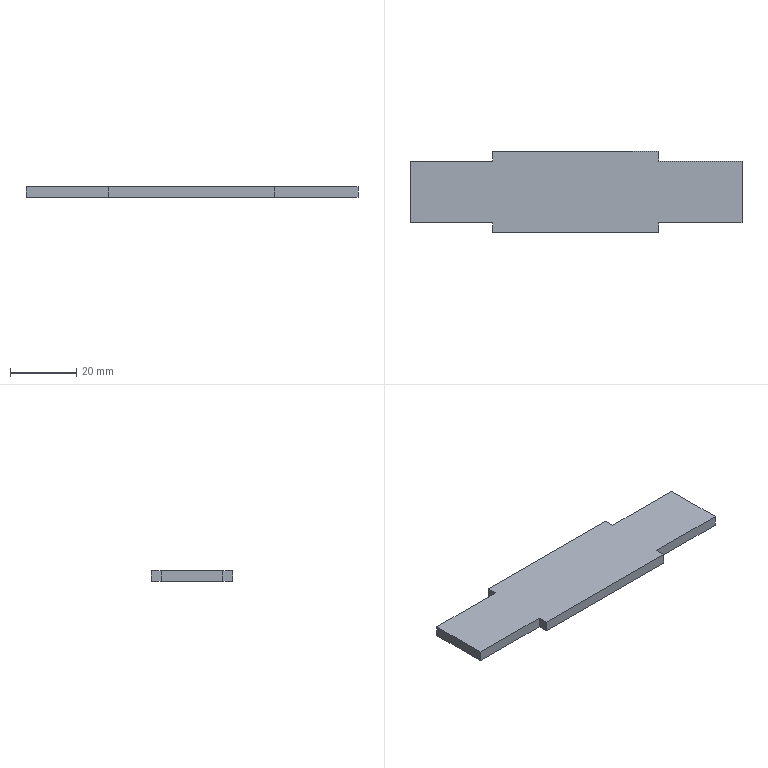Part | SolidWorks | features FlatPattern 1, SMBaseFlange 1, SheetMetal 1 | 1 solid | 14 faces | box 100 x 24.6 x 3.2 mm | volume 6912 mm3 | plane 14
STEP:
#1=CARTESIAN_POINT('',(-70.,-18.6,0.));
#2=VERTEX_POINT('',#1);
#3=CARTESIAN_POINT('',(-70.,0.,0.));
#4=VERTEX_POINT('',#3);
#5=CARTESIAN_POINT('',(-70.,0.,0.));
#6=DIRECTION('',(0.,1.,0.));
#7=VECTOR('',#6,1000.);
#8=LINE('',#5,#7);
#9=EDGE_CURVE('',#2,#4,#8,.T.);
#10=ORIENTED_EDGE('',*,*,#9,.F.);
#11=CARTESIAN_POINT('',(-70.,-18.6,-3.2));
#12=VERTEX_POINT('',#11);
#13=CARTESIAN_POINT('',(-70.,-18.6,-3.2));
#14=DIRECTION('',(0.,0.,1.));
#15=VECTOR('',#14,1000.);
#16=LINE('',#13,#15);
#17=EDGE_CURVE('',#12,#2,#16,.T.);
#18=ORIENTED_EDGE('',*,*,#17,.F.);
#19=CARTESIAN_POINT('',(-70.,0.,-3.2));
#20=VERTEX_POINT('',#19);
#21=CARTESIAN_POINT('',(-70.,0.,-3.2));
#22=DIRECTION('',(0.,1.,0.));
#23=VECTOR('',#22,1000.);
#24=LINE('',#21,#23);
#25=EDGE_CURVE('',#12,#20,#24,.T.);
#26=ORIENTED_EDGE('',*,*,#25,.T.);
#27=CARTESIAN_POINT('',(-70.,0.,-3.2));
#28=DIRECTION('',(0.,0.,1.));
#29=VECTOR('',#28,1000.);
#30=LINE('',#27,#29);
#31=EDGE_CURVE('',#20,#4,#30,.T.);
#32=ORIENTED_EDGE('',*,*,#31,.T.);
#33=EDGE_LOOP('',(#10,#18,#26,#32));
#34=FACE_OUTER_BOUND('',#33,.T.);
#35=CARTESIAN_POINT('',(-70.,0.,-3.2));
#36=DIRECTION('',(1.,0.,0.));
#37=DIRECTION('',(0.,0.,-1.));
#38=AXIS2_PLACEMENT_3D('',#35,#36,#37);
#39=PLANE('',#38);
#40=ADVANCED_FACE('',(#34),#39,.T.);
#41=CARTESIAN_POINT('',(-95.,-18.6,0.));
#42=VERTEX_POINT('',#41);
#43=CARTESIAN_POINT('',(-70.,-18.6,0.));
#44=DIRECTION('',(1.,0.,0.));
#45=VECTOR('',#44,1000.);
#46=LINE('',#43,#45);
#47=EDGE_CURVE('',#42,#2,#46,.T.);
#48=ORIENTED_EDGE('',*,*,#47,.F.);
#49=CARTESIAN_POINT('',(-95.,-18.6,-3.2));
#50=VERTEX_POINT('',#49);
#51=CARTESIAN_POINT('',(-95.,-18.6,-3.2));
#52=DIRECTION('',(0.,0.,1.));
#53=VECTOR('',#52,1000.);
#54=LINE('',#51,#53);
#55=EDGE_CURVE('',#50,#42,#54,.T.);
#56=ORIENTED_EDGE('',*,*,#55,.F.);
#57=CARTESIAN_POINT('',(-70.,-18.6,-3.2));
#58=DIRECTION('',(1.,0.,0.));
#59=VECTOR('',#58,1000.);
#60=LINE('',#57,#59);
#61=EDGE_CURVE('',#50,#12,#60,.T.);
#62=ORIENTED_EDGE('',*,*,#61,.T.);
#63=ORIENTED_EDGE('',*,*,#17,.T.);
#64=EDGE_LOOP('',(#48,#56,#62,#63));
#65=FACE_OUTER_BOUND('',#64,.T.);
#66=CARTESIAN_POINT('',(-70.,-18.6,-3.2));
#67=DIRECTION('',(0.,-1.,0.));
#68=DIRECTION('',(1.,0.,0.));
#69=AXIS2_PLACEMENT_3D('',#66,#67,#68);
#70=PLANE('',#69);
#71=ADVANCED_FACE('',(#65),#70,.T.);
#72=CARTESIAN_POINT('',(-95.,-21.6,0.));
#73=VERTEX_POINT('',#72);
#74=CARTESIAN_POINT('',(-95.,-18.6,0.));
#75=DIRECTION('',(0.,1.,0.));
#76=VECTOR('',#75,1000.);
#77=LINE('',#74,#76);
#78=EDGE_CURVE('',#73,#42,#77,.T.);
#79=ORIENTED_EDGE('',*,*,#78,.F.);
#80=CARTESIAN_POINT('',(-95.,-21.6,-3.2));
#81=VERTEX_POINT('',#80);
#82=CARTESIAN_POINT('',(-95.,-21.6,-3.2));
#83=DIRECTION('',(0.,0.,1.));
#84=VECTOR('',#83,1000.);
#85=LINE('',#82,#84);
#86=EDGE_CURVE('',#81,#73,#85,.T.);
#87=ORIENTED_EDGE('',*,*,#86,.F.);
#88=CARTESIAN_POINT('',(-95.,-18.6,-3.2));
#89=DIRECTION('',(0.,1.,0.));
#90=VECTOR('',#89,1000.);
#91=LINE('',#88,#90);
#92=EDGE_CURVE('',#81,#50,#91,.T.);
#93=ORIENTED_EDGE('',*,*,#92,.T.);
#94=ORIENTED_EDGE('',*,*,#55,.T.);
#95=EDGE_LOOP('',(#79,#87,#93,#94));
#96=FACE_OUTER_BOUND('',#95,.T.);
#97=CARTESIAN_POINT('',(-95.,-18.6,-3.2));
#98=DIRECTION('',(1.,0.,0.));
#99=DIRECTION('',(0.,0.,-1.));
#100=AXIS2_PLACEMENT_3D('',#97,#98,#99);
#101=PLANE('',#100);
#102=ADVANCED_FACE('',(#96),#101,.T.);
#103=CARTESIAN_POINT('',(-145.,-21.6,0.));
#104=VERTEX_POINT('',#103);
#105=CARTESIAN_POINT('',(-95.,-21.6,0.));
#106=DIRECTION('',(1.,0.,0.));
#107=VECTOR('',#106,1000.);
#108=LINE('',#105,#107);
#109=EDGE_CURVE('',#104,#73,#108,.T.);
#110=ORIENTED_EDGE('',*,*,#109,.F.);
#111=CARTESIAN_POINT('',(-145.,-21.6,-3.2));
#112=VERTEX_POINT('',#111);
#113=CARTESIAN_POINT('',(-145.,-21.6,-3.2));
#114=DIRECTION('',(0.,0.,1.));
#115=VECTOR('',#114,1000.);
#116=LINE('',#113,#115);
#117=EDGE_CURVE('',#112,#104,#116,.T.);
#118=ORIENTED_EDGE('',*,*,#117,.F.);
#119=CARTESIAN_POINT('',(-95.,-21.6,-3.2));
#120=DIRECTION('',(1.,0.,0.));
#121=VECTOR('',#120,1000.);
#122=LINE('',#119,#121);
#123=EDGE_CURVE('',#112,#81,#122,.T.);
#124=ORIENTED_EDGE('',*,*,#123,.T.);
#125=ORIENTED_EDGE('',*,*,#86,.T.);
#126=EDGE_LOOP('',(#110,#118,#124,#125));
#127=FACE_OUTER_BOUND('',#126,.T.);
#128=CARTESIAN_POINT('',(-95.,-21.6,-3.2));
#129=DIRECTION('',(0.,-1.,0.));
#130=DIRECTION('',(1.,0.,0.));
#131=AXIS2_PLACEMENT_3D('',#128,#129,#130);
#132=PLANE('',#131);
#133=ADVANCED_FACE('',(#127),#132,.T.);
#134=CARTESIAN_POINT('',(-145.,-18.6,0.));
#135=VERTEX_POINT('',#134);
#136=CARTESIAN_POINT('',(-145.,-21.6,0.));
#137=DIRECTION('',(0.,-1.,0.));
#138=VECTOR('',#137,1000.);
#139=LINE('',#136,#138);
#140=EDGE_CURVE('',#135,#104,#139,.T.);
#141=ORIENTED_EDGE('',*,*,#140,.F.);
#142=CARTESIAN_POINT('',(-145.,-18.6,-3.2));
#143=VERTEX_POINT('',#142);
#144=CARTESIAN_POINT('',(-145.,-18.6,-3.2));
#145=DIRECTION('',(0.,0.,1.));
#146=VECTOR('',#145,1000.);
#147=LINE('',#144,#146);
#148=EDGE_CURVE('',#143,#135,#147,.T.);
#149=ORIENTED_EDGE('',*,*,#148,.F.);
#150=CARTESIAN_POINT('',(-145.,-21.6,-3.2));
#151=DIRECTION('',(0.,-1.,0.));
#152=VECTOR('',#151,1000.);
#153=LINE('',#150,#152);
#154=EDGE_CURVE('',#143,#112,#153,.T.);
#155=ORIENTED_EDGE('',*,*,#154,.T.);
#156=ORIENTED_EDGE('',*,*,#117,.T.);
#157=EDGE_LOOP('',(#141,#149,#155,#156));
#158=FACE_OUTER_BOUND('',#157,.T.);
#159=CARTESIAN_POINT('',(-145.,-21.6,-3.2));
#160=DIRECTION('',(-1.,0.,0.));
#161=DIRECTION('',(0.,0.,1.));
#162=AXIS2_PLACEMENT_3D('',#159,#160,#161);
#163=PLANE('',#162);
#164=ADVANCED_FACE('',(#158),#163,.T.);
#165=CARTESIAN_POINT('',(-170.,-18.6,0.));
#166=VERTEX_POINT('',#165);
#167=CARTESIAN_POINT('',(-145.,-18.6,0.));
#168=DIRECTION('',(1.,0.,0.));
#169=VECTOR('',#168,1000.);
#170=LINE('',#167,#169);
#171=EDGE_CURVE('',#166,#135,#170,.T.);
#172=ORIENTED_EDGE('',*,*,#171,.F.);
#173=CARTESIAN_POINT('',(-170.,-18.6,-3.2));
#174=VERTEX_POINT('',#173);
#175=CARTESIAN_POINT('',(-170.,-18.6,-3.2));
#176=DIRECTION('',(0.,0.,1.));
#177=VECTOR('',#176,1000.);
#178=LINE('',#175,#177);
#179=EDGE_CURVE('',#174,#166,#178,.T.);
#180=ORIENTED_EDGE('',*,*,#179,.F.);
#181=CARTESIAN_POINT('',(-145.,-18.6,-3.2));
#182=DIRECTION('',(1.,0.,0.));
#183=VECTOR('',#182,1000.);
#184=LINE('',#181,#183);
#185=EDGE_CURVE('',#174,#143,#184,.T.);
#186=ORIENTED_EDGE('',*,*,#185,.T.);
#187=ORIENTED_EDGE('',*,*,#148,.T.);
#188=EDGE_LOOP('',(#172,#180,#186,#187));
#189=FACE_OUTER_BOUND('',#188,.T.);
#190=CARTESIAN_POINT('',(-145.,-18.6,-3.2));
#191=DIRECTION('',(0.,-1.,0.));
#192=DIRECTION('',(1.,0.,0.));
#193=AXIS2_PLACEMENT_3D('',#190,#191,#192);
#194=PLANE('',#193);
#195=ADVANCED_FACE('',(#189),#194,.T.);
#196=CARTESIAN_POINT('',(-170.,0.,0.));
#197=VERTEX_POINT('',#196);
#198=CARTESIAN_POINT('',(-170.,0.,0.));
#199=DIRECTION('',(0.,-1.,0.));
#200=VECTOR('',#199,1000.);
#201=LINE('',#198,#200);
#202=EDGE_CURVE('',#197,#166,#201,.T.);
#203=ORIENTED_EDGE('',*,*,#202,.F.);
#204=CARTESIAN_POINT('',(-170.,0.,-3.2));
#205=VERTEX_POINT('',#204);
#206=CARTESIAN_POINT('',(-170.,0.,-3.2));
#207=DIRECTION('',(0.,0.,1.));
#208=VECTOR('',#207,1000.);
#209=LINE('',#206,#208);
#210=EDGE_CURVE('',#205,#197,#209,.T.);
#211=ORIENTED_EDGE('',*,*,#210,.F.);
#212=CARTESIAN_POINT('',(-170.,0.,-3.2));
#213=DIRECTION('',(0.,-1.,0.));
#214=VECTOR('',#213,1000.);
#215=LINE('',#212,#214);
#216=EDGE_CURVE('',#205,#174,#215,.T.);
#217=ORIENTED_EDGE('',*,*,#216,.T.);
#218=ORIENTED_EDGE('',*,*,#179,.T.);
#219=EDGE_LOOP('',(#203,#211,#217,#218));
#220=FACE_OUTER_BOUND('',#219,.T.);
#221=CARTESIAN_POINT('',(-170.,0.,-3.2));
#222=DIRECTION('',(-1.,0.,0.));
#223=DIRECTION('',(0.,0.,1.));
#224=AXIS2_PLACEMENT_3D('',#221,#222,#223);
#225=PLANE('',#224);
#226=ADVANCED_FACE('',(#220),#225,.T.);
#227=CARTESIAN_POINT('',(-145.,0.,0.));
#228=VERTEX_POINT('',#227);
#229=CARTESIAN_POINT('',(-145.,0.,0.));
#230=DIRECTION('',(-1.,0.,0.));
#231=VECTOR('',#230,1000.);
#232=LINE('',#229,#231);
#233=EDGE_CURVE('',#228,#197,#232,.T.);
#234=ORIENTED_EDGE('',*,*,#233,.F.);
#235=CARTESIAN_POINT('',(-145.,0.,-3.2));
#236=VERTEX_POINT('',#235);
#237=CARTESIAN_POINT('',(-145.,0.,-3.2));
#238=DIRECTION('',(0.,0.,1.));
#239=VECTOR('',#238,1000.);
#240=LINE('',#237,#239);
#241=EDGE_CURVE('',#236,#228,#240,.T.);
#242=ORIENTED_EDGE('',*,*,#241,.F.);
#243=CARTESIAN_POINT('',(-145.,0.,-3.2));
#244=DIRECTION('',(-1.,0.,0.));
#245=VECTOR('',#244,1000.);
#246=LINE('',#243,#245);
#247=EDGE_CURVE('',#236,#205,#246,.T.);
#248=ORIENTED_EDGE('',*,*,#247,.T.);
#249=ORIENTED_EDGE('',*,*,#210,.T.);
#250=EDGE_LOOP('',(#234,#242,#248,#249));
#251=FACE_OUTER_BOUND('',#250,.T.);
#252=CARTESIAN_POINT('',(-145.,0.,-3.2));
#253=DIRECTION('',(0.,1.,0.));
#254=DIRECTION('',(-1.,0.,0.));
#255=AXIS2_PLACEMENT_3D('',#252,#253,#254);
#256=PLANE('',#255);
#257=ADVANCED_FACE('',(#251),#256,.T.);
#258=CARTESIAN_POINT('',(-145.,3.,0.));
#259=VERTEX_POINT('',#258);
#260=CARTESIAN_POINT('',(-145.,3.,0.));
#261=DIRECTION('',(0.,-1.,0.));
#262=VECTOR('',#261,1000.);
#263=LINE('',#260,#262);
#264=EDGE_CURVE('',#259,#228,#263,.T.);
#265=ORIENTED_EDGE('',*,*,#264,.F.);
#266=CARTESIAN_POINT('',(-145.,3.,-3.2));
#267=VERTEX_POINT('',#266);
#268=CARTESIAN_POINT('',(-145.,3.,-3.2));
#269=DIRECTION('',(0.,0.,1.));
#270=VECTOR('',#269,1000.);
#271=LINE('',#268,#270);
#272=EDGE_CURVE('',#267,#259,#271,.T.);
#273=ORIENTED_EDGE('',*,*,#272,.F.);
#274=CARTESIAN_POINT('',(-145.,3.,-3.2));
#275=DIRECTION('',(0.,-1.,0.));
#276=VECTOR('',#275,1000.);
#277=LINE('',#274,#276);
#278=EDGE_CURVE('',#267,#236,#277,.T.);
#279=ORIENTED_EDGE('',*,*,#278,.T.);
#280=ORIENTED_EDGE('',*,*,#241,.T.);
#281=EDGE_LOOP('',(#265,#273,#279,#280));
#282=FACE_OUTER_BOUND('',#281,.T.);
#283=CARTESIAN_POINT('',(-145.,3.,-3.2));
#284=DIRECTION('',(-1.,0.,0.));
#285=DIRECTION('',(0.,0.,1.));
#286=AXIS2_PLACEMENT_3D('',#283,#284,#285);
#287=PLANE('',#286);
#288=ADVANCED_FACE('',(#282),#287,.T.);
#289=CARTESIAN_POINT('',(-95.,3.,0.));
#290=VERTEX_POINT('',#289);
#291=CARTESIAN_POINT('',(-95.,3.,0.));
#292=DIRECTION('',(-1.,0.,0.));
#293=VECTOR('',#292,1000.);
#294=LINE('',#291,#293);
#295=EDGE_CURVE('',#290,#259,#294,.T.);
#296=ORIENTED_EDGE('',*,*,#295,.F.);
#297=CARTESIAN_POINT('',(-95.,3.,-3.2));
#298=VERTEX_POINT('',#297);
#299=CARTESIAN_POINT('',(-95.,3.,-3.2));
#300=DIRECTION('',(0.,0.,1.));
#301=VECTOR('',#300,1000.);
#302=LINE('',#299,#301);
#303=EDGE_CURVE('',#298,#290,#302,.T.);
#304=ORIENTED_EDGE('',*,*,#303,.F.);
#305=CARTESIAN_POINT('',(-95.,3.,-3.2));
#306=DIRECTION('',(-1.,0.,0.));
#307=VECTOR('',#306,1000.);
#308=LINE('',#305,#307);
#309=EDGE_CURVE('',#298,#267,#308,.T.);
#310=ORIENTED_EDGE('',*,*,#309,.T.);
#311=ORIENTED_EDGE('',*,*,#272,.T.);
#312=EDGE_LOOP('',(#296,#304,#310,#311));
#313=FACE_OUTER_BOUND('',#312,.T.);
#314=CARTESIAN_POINT('',(-95.,3.,-3.2));
#315=DIRECTION('',(0.,1.,0.));
#316=DIRECTION('',(-1.,0.,0.));
#317=AXIS2_PLACEMENT_3D('',#314,#315,#316);
#318=PLANE('',#317);
#319=ADVANCED_FACE('',(#313),#318,.T.);
#320=CARTESIAN_POINT('',(-95.,0.,0.));
#321=VERTEX_POINT('',#320);
#322=CARTESIAN_POINT('',(-95.,0.,0.));
#323=DIRECTION('',(0.,1.,0.));
#324=VECTOR('',#323,1000.);
#325=LINE('',#322,#324);
#326=EDGE_CURVE('',#321,#290,#325,.T.);
#327=ORIENTED_EDGE('',*,*,#326,.F.);
#328=CARTESIAN_POINT('',(-95.,0.,-3.2));
#329=VERTEX_POINT('',#328);
#330=CARTESIAN_POINT('',(-95.,0.,-3.2));
#331=DIRECTION('',(0.,0.,1.));
#332=VECTOR('',#331,1000.);
#333=LINE('',#330,#332);
#334=EDGE_CURVE('',#329,#321,#333,.T.);
#335=ORIENTED_EDGE('',*,*,#334,.F.);
#336=CARTESIAN_POINT('',(-95.,0.,-3.2));
#337=DIRECTION('',(0.,1.,0.));
#338=VECTOR('',#337,1000.);
#339=LINE('',#336,#338);
#340=EDGE_CURVE('',#329,#298,#339,.T.);
#341=ORIENTED_EDGE('',*,*,#340,.T.);
#342=ORIENTED_EDGE('',*,*,#303,.T.);
#343=EDGE_LOOP('',(#327,#335,#341,#342));
#344=FACE_OUTER_BOUND('',#343,.T.);
#345=CARTESIAN_POINT('',(-95.,0.,-3.2));
#346=DIRECTION('',(1.,0.,0.));
#347=DIRECTION('',(0.,0.,-1.));
#348=AXIS2_PLACEMENT_3D('',#345,#346,#347);
#349=PLANE('',#348);
#350=ADVANCED_FACE('',(#344),#349,.T.);
#351=CARTESIAN_POINT('',(-70.,0.,0.));
#352=DIRECTION('',(-1.,0.,0.));
#353=VECTOR('',#352,1000.);
#354=LINE('',#351,#353);
#355=EDGE_CURVE('',#4,#321,#354,.T.);
#356=ORIENTED_EDGE('',*,*,#355,.F.);
#357=ORIENTED_EDGE('',*,*,#31,.F.);
#358=CARTESIAN_POINT('',(-70.,0.,-3.2));
#359=DIRECTION('',(-1.,0.,0.));
#360=VECTOR('',#359,1000.);
#361=LINE('',#358,#360);
#362=EDGE_CURVE('',#20,#329,#361,.T.);
#363=ORIENTED_EDGE('',*,*,#362,.T.);
#364=ORIENTED_EDGE('',*,*,#334,.T.);
#365=EDGE_LOOP('',(#356,#357,#363,#364));
#366=FACE_OUTER_BOUND('',#365,.T.);
#367=CARTESIAN_POINT('',(-70.,0.,-3.2));
#368=DIRECTION('',(0.,1.,0.));
#369=DIRECTION('',(-1.,0.,0.));
#370=AXIS2_PLACEMENT_3D('',#367,#368,#369);
#371=PLANE('',#370);
#372=ADVANCED_FACE('',(#366),#371,.T.);
#373=ORIENTED_EDGE('',*,*,#25,.F.);
#374=ORIENTED_EDGE('',*,*,#61,.F.);
#375=ORIENTED_EDGE('',*,*,#92,.F.);
#376=ORIENTED_EDGE('',*,*,#123,.F.);
#377=ORIENTED_EDGE('',*,*,#154,.F.);
#378=ORIENTED_EDGE('',*,*,#185,.F.);
#379=ORIENTED_EDGE('',*,*,#216,.F.);
#380=ORIENTED_EDGE('',*,*,#247,.F.);
#381=ORIENTED_EDGE('',*,*,#278,.F.);
#382=ORIENTED_EDGE('',*,*,#309,.F.);
#383=ORIENTED_EDGE('',*,*,#340,.F.);
#384=ORIENTED_EDGE('',*,*,#362,.F.);
#385=EDGE_LOOP('',(#373,#374,#375,#376,#377,#378,#379,#380,#381,#382,#383,#384));
#386=FACE_OUTER_BOUND('',#385,.T.);
#387=CARTESIAN_POINT('',(0.,0.,-3.2));
#388=DIRECTION('',(0.,0.,-1.));
#389=DIRECTION('',(-1.,0.,0.));
#390=AXIS2_PLACEMENT_3D('',#387,#388,#389);
#391=PLANE('',#390);
#392=ADVANCED_FACE('',(#386),#391,.T.);
#393=ORIENTED_EDGE('',*,*,#9,.T.);
#394=ORIENTED_EDGE('',*,*,#355,.T.);
#395=ORIENTED_EDGE('',*,*,#326,.T.);
#396=ORIENTED_EDGE('',*,*,#295,.T.);
#397=ORIENTED_EDGE('',*,*,#264,.T.);
#398=ORIENTED_EDGE('',*,*,#233,.T.);
#399=ORIENTED_EDGE('',*,*,#202,.T.);
#400=ORIENTED_EDGE('',*,*,#171,.T.);
#401=ORIENTED_EDGE('',*,*,#140,.T.);
#402=ORIENTED_EDGE('',*,*,#109,.T.);
#403=ORIENTED_EDGE('',*,*,#78,.T.);
#404=ORIENTED_EDGE('',*,*,#47,.T.);
#405=EDGE_LOOP('',(#393,#394,#395,#396,#397,#398,#399,#400,#401,#402,#403,#404));
#406=FACE_OUTER_BOUND('',#405,.T.);
#407=CARTESIAN_POINT('',(0.,0.,0.));
#408=DIRECTION('',(0.,0.,-1.));
#409=DIRECTION('',(-1.,0.,0.));
#410=AXIS2_PLACEMENT_3D('',#407,#408,#409);
#411=PLANE('',#410);
#412=ADVANCED_FACE('',(#406),#411,.F.);
#413=CLOSED_SHELL('',(#40,#71,#102,#133,#164,#195,#226,#257,#288,#319,#350,#372,#392,#412));
#414=MANIFOLD_SOLID_BREP('',#413);
#415=CARTESIAN_POINT('',(0.,0.,0.));
#416=DIRECTION('',(0.,0.,1.));
#417=DIRECTION('',(1.,0.,0.));
#418=AXIS2_PLACEMENT_3D('',#415,#416,#417);
#419=(LENGTH_UNIT()NAMED_UNIT(*)SI_UNIT(.MILLI.,.METRE.));
#420=UNCERTAINTY_MEASURE_WITH_UNIT(LENGTH_MEASURE(0.00001),#419,'','');
#421=(NAMED_UNIT(*)PLANE_ANGLE_UNIT()SI_UNIT($,.RADIAN.));
#422=(NAMED_UNIT(*)SI_UNIT($,.STERADIAN.)SOLID_ANGLE_UNIT());
#423=(GEOMETRIC_REPRESENTATION_CONTEXT(3)GLOBAL_UNCERTAINTY_ASSIGNED_CONTEXT((#420))GLOBAL_UNIT_ASSIGNED_CONTEXT((#419,#421,#422))REPRESENTATION_CONTEXT('',''));
#424=ADVANCED_BREP_SHAPE_REPRESENTATION('',(#414,#418),#423);